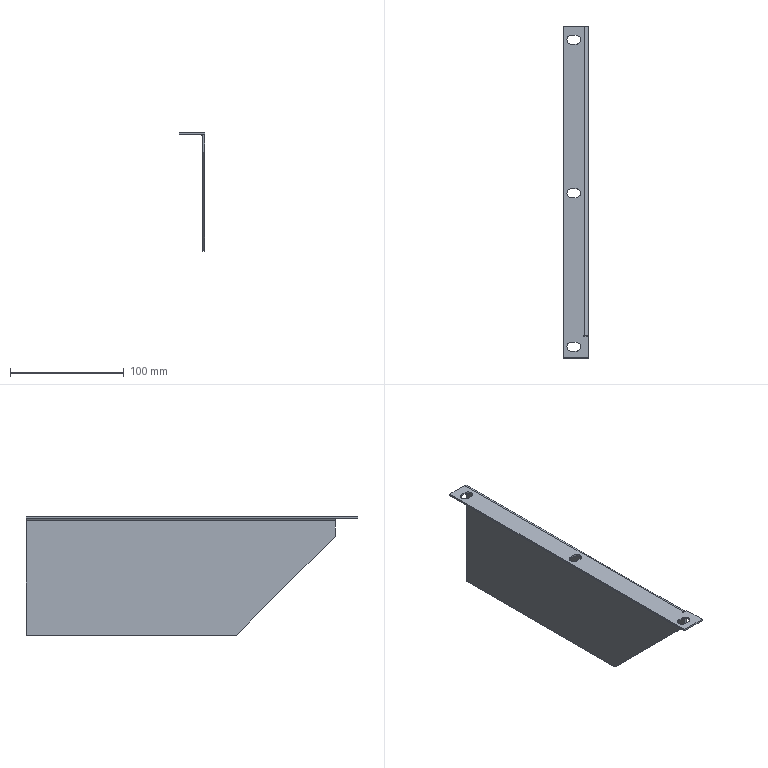Part | STEP file | SYL_0392D6J1SYL0380DJ100-657963 | 1 solid | 37 faces | box 22 x 292 x 104 mm | volume 44923 mm3 | plane 23 | cylinder 14 | commonest cylinder face diameters 8 x12 4 x1 7 x1
STEP:
#1=CARTESIAN_POINT('',(-13.5,120.,0.));
#2=VERTEX_POINT('',#1);
#3=CARTESIAN_POINT('',(-13.5,120.,-1.5));
#4=VERTEX_POINT('',#3);
#5=CARTESIAN_POINT('',(-13.5,120.,-1.5));
#6=DIRECTION('',(0.,0.,-1.));
#7=VECTOR('',#6,1000.);
#8=LINE('',#5,#7);
#9=EDGE_CURVE('',#2,#4,#8,.T.);
#10=ORIENTED_EDGE('',*,*,#9,.F.);
#11=CARTESIAN_POINT('',(-9.5,120.,0.));
#12=VERTEX_POINT('',#11);
#13=CARTESIAN_POINT('',(1.5,120.,0.));
#14=DIRECTION('',(1.,0.,0.));
#15=VECTOR('',#14,1000.);
#16=LINE('',#13,#15);
#17=EDGE_CURVE('',#2,#12,#16,.T.);
#18=ORIENTED_EDGE('',*,*,#17,.T.);
#19=CARTESIAN_POINT('',(-9.5,120.,-1.5));
#20=VERTEX_POINT('',#19);
#21=CARTESIAN_POINT('',(-9.5,120.,-1.5));
#22=DIRECTION('',(0.,0.,-1.));
#23=VECTOR('',#22,1000.);
#24=LINE('',#21,#23);
#25=EDGE_CURVE('',#12,#20,#24,.T.);
#26=ORIENTED_EDGE('',*,*,#25,.T.);
#27=CARTESIAN_POINT('',(-13.5,120.,-1.5));
#28=DIRECTION('',(1.,0.,0.));
#29=VECTOR('',#28,1000.);
#30=LINE('',#27,#29);
#31=EDGE_CURVE('',#4,#20,#30,.T.);
#32=ORIENTED_EDGE('',*,*,#31,.F.);
#33=EDGE_LOOP('',(#10,#18,#26,#32));
#34=FACE_OUTER_BOUND('',#33,.T.);
#35=CARTESIAN_POINT('',(-13.5,120.,-1.5));
#36=DIRECTION('',(0.,-1.,0.));
#37=DIRECTION('',(1.,0.,0.));
#38=AXIS2_PLACEMENT_3D('',#35,#36,#37);
#39=PLANE('',#38);
#40=ADVANCED_FACE('',(#34),#39,.F.);
#41=ORIENTED_EDGE('',*,*,#25,.F.);
#42=CARTESIAN_POINT('',(-5.5,124.,0.));
#43=VERTEX_POINT('',#42);
#44=CARTESIAN_POINT('',(-9.5,124.,0.));
#45=DIRECTION('',(0.,0.,1.));
#46=DIRECTION('',(1.,0.,0.));
#47=AXIS2_PLACEMENT_3D('',#44,#45,#46);
#48=CIRCLE('',#47,4.);
#49=EDGE_CURVE('',#12,#43,#48,.T.);
#50=ORIENTED_EDGE('',*,*,#49,.T.);
#51=CARTESIAN_POINT('',(-5.5,124.,-1.5));
#52=VERTEX_POINT('',#51);
#53=CARTESIAN_POINT('',(-5.5,124.,-1.5));
#54=DIRECTION('',(0.,0.,-1.));
#55=VECTOR('',#54,1000.);
#56=LINE('',#53,#55);
#57=EDGE_CURVE('',#43,#52,#56,.T.);
#58=ORIENTED_EDGE('',*,*,#57,.T.);
#59=CARTESIAN_POINT('',(-9.5,124.,-1.5));
#60=DIRECTION('',(0.,0.,1.));
#61=DIRECTION('',(0.,-1.,0.));
#62=AXIS2_PLACEMENT_3D('',#59,#60,#61);
#63=CIRCLE('',#62,4.);
#64=EDGE_CURVE('',#20,#52,#63,.T.);
#65=ORIENTED_EDGE('',*,*,#64,.F.);
#66=EDGE_LOOP('',(#41,#50,#58,#65));
#67=FACE_OUTER_BOUND('',#66,.T.);
#68=CARTESIAN_POINT('',(-9.5,124.,-1.5));
#69=DIRECTION('',(0.,0.,1.));
#70=DIRECTION('',(1.,0.,0.));
#71=AXIS2_PLACEMENT_3D('',#68,#69,#70);
#72=CYLINDRICAL_SURFACE('',#71,4.);
#73=ADVANCED_FACE('',(#67),#72,.F.);
#74=ORIENTED_EDGE('',*,*,#57,.F.);
#75=CARTESIAN_POINT('',(-9.5,128.,0.));
#76=VERTEX_POINT('',#75);
#77=CARTESIAN_POINT('',(-9.5,124.,0.));
#78=DIRECTION('',(0.,0.,1.));
#79=DIRECTION('',(1.,0.,0.));
#80=AXIS2_PLACEMENT_3D('',#77,#78,#79);
#81=CIRCLE('',#80,4.);
#82=EDGE_CURVE('',#43,#76,#81,.T.);
#83=ORIENTED_EDGE('',*,*,#82,.T.);
#84=CARTESIAN_POINT('',(-9.5,128.,-1.5));
#85=VERTEX_POINT('',#84);
#86=CARTESIAN_POINT('',(-9.5,128.,-1.5));
#87=DIRECTION('',(0.,0.,-1.));
#88=VECTOR('',#87,1000.);
#89=LINE('',#86,#88);
#90=EDGE_CURVE('',#76,#85,#89,.T.);
#91=ORIENTED_EDGE('',*,*,#90,.T.);
#92=CARTESIAN_POINT('',(-9.5,124.,-1.5));
#93=DIRECTION('',(0.,0.,1.));
#94=DIRECTION('',(1.,0.,0.));
#95=AXIS2_PLACEMENT_3D('',#92,#93,#94);
#96=CIRCLE('',#95,4.);
#97=EDGE_CURVE('',#52,#85,#96,.T.);
#98=ORIENTED_EDGE('',*,*,#97,.F.);
#99=EDGE_LOOP('',(#74,#83,#91,#98));
#100=FACE_OUTER_BOUND('',#99,.T.);
#101=CARTESIAN_POINT('',(-9.5,124.,-1.5));
#102=DIRECTION('',(0.,0.,1.));
#103=DIRECTION('',(1.,0.,0.));
#104=AXIS2_PLACEMENT_3D('',#101,#102,#103);
#105=CYLINDRICAL_SURFACE('',#104,4.);
#106=ADVANCED_FACE('',(#100),#105,.F.);
#107=ORIENTED_EDGE('',*,*,#90,.F.);
#108=CARTESIAN_POINT('',(-13.5,128.,0.));
#109=VERTEX_POINT('',#108);
#110=CARTESIAN_POINT('',(1.5,128.,0.));
#111=DIRECTION('',(-1.,0.,0.));
#112=VECTOR('',#111,1000.);
#113=LINE('',#110,#112);
#114=EDGE_CURVE('',#76,#109,#113,.T.);
#115=ORIENTED_EDGE('',*,*,#114,.T.);
#116=CARTESIAN_POINT('',(-13.5,128.,-1.5));
#117=VERTEX_POINT('',#116);
#118=CARTESIAN_POINT('',(-13.5,128.,-1.5));
#119=DIRECTION('',(0.,0.,-1.));
#120=VECTOR('',#119,1000.);
#121=LINE('',#118,#120);
#122=EDGE_CURVE('',#109,#117,#121,.T.);
#123=ORIENTED_EDGE('',*,*,#122,.T.);
#124=CARTESIAN_POINT('',(-9.5,128.,-1.5));
#125=DIRECTION('',(-1.,0.,0.));
#126=VECTOR('',#125,1000.);
#127=LINE('',#124,#126);
#128=EDGE_CURVE('',#85,#117,#127,.T.);
#129=ORIENTED_EDGE('',*,*,#128,.F.);
#130=EDGE_LOOP('',(#107,#115,#123,#129));
#131=FACE_OUTER_BOUND('',#130,.T.);
#132=CARTESIAN_POINT('',(-9.5,128.,-1.5));
#133=DIRECTION('',(0.,1.,0.));
#134=DIRECTION('',(-1.,0.,0.));
#135=AXIS2_PLACEMENT_3D('',#132,#133,#134);
#136=PLANE('',#135);
#137=ADVANCED_FACE('',(#131),#136,.F.);
#138=ORIENTED_EDGE('',*,*,#122,.F.);
#139=CARTESIAN_POINT('',(-17.5,124.,0.));
#140=VERTEX_POINT('',#139);
#141=CARTESIAN_POINT('',(-13.5,124.,0.));
#142=DIRECTION('',(0.,0.,1.));
#143=DIRECTION('',(1.,0.,0.));
#144=AXIS2_PLACEMENT_3D('',#141,#142,#143);
#145=CIRCLE('',#144,4.);
#146=EDGE_CURVE('',#109,#140,#145,.T.);
#147=ORIENTED_EDGE('',*,*,#146,.T.);
#148=CARTESIAN_POINT('',(-17.5,124.,-1.5));
#149=VERTEX_POINT('',#148);
#150=CARTESIAN_POINT('',(-17.5,124.,-1.5));
#151=DIRECTION('',(0.,0.,-1.));
#152=VECTOR('',#151,1000.);
#153=LINE('',#150,#152);
#154=EDGE_CURVE('',#140,#149,#153,.T.);
#155=ORIENTED_EDGE('',*,*,#154,.T.);
#156=CARTESIAN_POINT('',(-13.5,124.,-1.5));
#157=DIRECTION('',(0.,0.,1.));
#158=DIRECTION('',(0.,1.,0.));
#159=AXIS2_PLACEMENT_3D('',#156,#157,#158);
#160=CIRCLE('',#159,4.);
#161=EDGE_CURVE('',#117,#149,#160,.T.);
#162=ORIENTED_EDGE('',*,*,#161,.F.);
#163=EDGE_LOOP('',(#138,#147,#155,#162));
#164=FACE_OUTER_BOUND('',#163,.T.);
#165=CARTESIAN_POINT('',(-13.5,124.,-1.5));
#166=DIRECTION('',(0.,0.,1.));
#167=DIRECTION('',(1.,0.,0.));
#168=AXIS2_PLACEMENT_3D('',#165,#166,#167);
#169=CYLINDRICAL_SURFACE('',#168,4.);
#170=ADVANCED_FACE('',(#164),#169,.F.);
#171=CARTESIAN_POINT('',(-13.5,-15.,0.));
#172=VERTEX_POINT('',#171);
#173=CARTESIAN_POINT('',(-13.5,-15.,-1.5));
#174=VERTEX_POINT('',#173);
#175=CARTESIAN_POINT('',(-13.5,-15.,-1.5));
#176=DIRECTION('',(0.,0.,-1.));
#177=VECTOR('',#176,1000.);
#178=LINE('',#175,#177);
#179=EDGE_CURVE('',#172,#174,#178,.T.);
#180=ORIENTED_EDGE('',*,*,#179,.F.);
#181=CARTESIAN_POINT('',(-9.5,-15.,0.));
#182=VERTEX_POINT('',#181);
#183=CARTESIAN_POINT('',(1.5,-15.,0.));
#184=DIRECTION('',(1.,0.,0.));
#185=VECTOR('',#184,1000.);
#186=LINE('',#183,#185);
#187=EDGE_CURVE('',#172,#182,#186,.T.);
#188=ORIENTED_EDGE('',*,*,#187,.T.);
#189=CARTESIAN_POINT('',(-9.5,-15.,-1.5));
#190=VERTEX_POINT('',#189);
#191=CARTESIAN_POINT('',(-9.5,-15.,-1.5));
#192=DIRECTION('',(0.,0.,-1.));
#193=VECTOR('',#192,1000.);
#194=LINE('',#191,#193);
#195=EDGE_CURVE('',#182,#190,#194,.T.);
#196=ORIENTED_EDGE('',*,*,#195,.T.);
#197=CARTESIAN_POINT('',(-13.5,-15.,-1.5));
#198=DIRECTION('',(1.,0.,0.));
#199=VECTOR('',#198,1000.);
#200=LINE('',#197,#199);
#201=EDGE_CURVE('',#174,#190,#200,.T.);
#202=ORIENTED_EDGE('',*,*,#201,.F.);
#203=EDGE_LOOP('',(#180,#188,#196,#202));
#204=FACE_OUTER_BOUND('',#203,.T.);
#205=CARTESIAN_POINT('',(-13.5,-15.,-1.5));
#206=DIRECTION('',(0.,-1.,0.));
#207=DIRECTION('',(1.,0.,0.));
#208=AXIS2_PLACEMENT_3D('',#205,#206,#207);
#209=PLANE('',#208);
#210=ADVANCED_FACE('',(#204),#209,.F.);
#211=ORIENTED_EDGE('',*,*,#195,.F.);
#212=CARTESIAN_POINT('',(-5.5,-11.,0.));
#213=VERTEX_POINT('',#212);
#214=CARTESIAN_POINT('',(-9.5,-11.,0.));
#215=DIRECTION('',(0.,0.,1.));
#216=DIRECTION('',(1.,0.,0.));
#217=AXIS2_PLACEMENT_3D('',#214,#215,#216);
#218=CIRCLE('',#217,4.);
#219=EDGE_CURVE('',#182,#213,#218,.T.);
#220=ORIENTED_EDGE('',*,*,#219,.T.);
#221=CARTESIAN_POINT('',(-5.5,-11.,-1.5));
#222=VERTEX_POINT('',#221);
#223=CARTESIAN_POINT('',(-5.5,-11.,-1.5));
#224=DIRECTION('',(0.,0.,-1.));
#225=VECTOR('',#224,1000.);
#226=LINE('',#223,#225);
#227=EDGE_CURVE('',#213,#222,#226,.T.);
#228=ORIENTED_EDGE('',*,*,#227,.T.);
#229=CARTESIAN_POINT('',(-9.5,-11.,-1.5));
#230=DIRECTION('',(0.,0.,1.));
#231=DIRECTION('',(0.,-1.,0.));
#232=AXIS2_PLACEMENT_3D('',#229,#230,#231);
#233=CIRCLE('',#232,4.);
#234=EDGE_CURVE('',#190,#222,#233,.T.);
#235=ORIENTED_EDGE('',*,*,#234,.F.);
#236=EDGE_LOOP('',(#211,#220,#228,#235));
#237=FACE_OUTER_BOUND('',#236,.T.);
#238=CARTESIAN_POINT('',(-9.5,-11.,-1.5));
#239=DIRECTION('',(0.,0.,1.));
#240=DIRECTION('',(1.,0.,0.));
#241=AXIS2_PLACEMENT_3D('',#238,#239,#240);
#242=CYLINDRICAL_SURFACE('',#241,4.);
#243=ADVANCED_FACE('',(#237),#242,.F.);
#244=ORIENTED_EDGE('',*,*,#227,.F.);
#245=CARTESIAN_POINT('',(-9.5,-7.,0.));
#246=VERTEX_POINT('',#245);
#247=CARTESIAN_POINT('',(-9.5,-11.,0.));
#248=DIRECTION('',(0.,0.,1.));
#249=DIRECTION('',(1.,0.,0.));
#250=AXIS2_PLACEMENT_3D('',#247,#248,#249);
#251=CIRCLE('',#250,4.);
#252=EDGE_CURVE('',#213,#246,#251,.T.);
#253=ORIENTED_EDGE('',*,*,#252,.T.);
#254=CARTESIAN_POINT('',(-9.5,-7.,-1.5));
#255=VERTEX_POINT('',#254);
#256=CARTESIAN_POINT('',(-9.5,-7.,-1.5));
#257=DIRECTION('',(0.,0.,-1.));
#258=VECTOR('',#257,1000.);
#259=LINE('',#256,#258);
#260=EDGE_CURVE('',#246,#255,#259,.T.);
#261=ORIENTED_EDGE('',*,*,#260,.T.);
#262=CARTESIAN_POINT('',(-9.5,-11.,-1.5));
#263=DIRECTION('',(0.,0.,1.));
#264=DIRECTION('',(1.,0.,0.));
#265=AXIS2_PLACEMENT_3D('',#262,#263,#264);
#266=CIRCLE('',#265,4.);
#267=EDGE_CURVE('',#222,#255,#266,.T.);
#268=ORIENTED_EDGE('',*,*,#267,.F.);
#269=EDGE_LOOP('',(#244,#253,#261,#268));
#270=FACE_OUTER_BOUND('',#269,.T.);
#271=CARTESIAN_POINT('',(-9.5,-11.,-1.5));
#272=DIRECTION('',(0.,0.,1.));
#273=DIRECTION('',(1.,0.,0.));
#274=AXIS2_PLACEMENT_3D('',#271,#272,#273);
#275=CYLINDRICAL_SURFACE('',#274,4.);
#276=ADVANCED_FACE('',(#270),#275,.F.);
#277=ORIENTED_EDGE('',*,*,#260,.F.);
#278=CARTESIAN_POINT('',(-13.5,-7.,0.));
#279=VERTEX_POINT('',#278);
#280=CARTESIAN_POINT('',(1.5,-7.,0.));
#281=DIRECTION('',(-1.,0.,0.));
#282=VECTOR('',#281,1000.);
#283=LINE('',#280,#282);
#284=EDGE_CURVE('',#246,#279,#283,.T.);
#285=ORIENTED_EDGE('',*,*,#284,.T.);
#286=CARTESIAN_POINT('',(-13.5,-7.,-1.5));
#287=VERTEX_POINT('',#286);
#288=CARTESIAN_POINT('',(-13.5,-7.,-1.5));
#289=DIRECTION('',(0.,0.,-1.));
#290=VECTOR('',#289,1000.);
#291=LINE('',#288,#290);
#292=EDGE_CURVE('',#279,#287,#291,.T.);
#293=ORIENTED_EDGE('',*,*,#292,.T.);
#294=CARTESIAN_POINT('',(-9.5,-7.,-1.5));
#295=DIRECTION('',(-1.,0.,0.));
#296=VECTOR('',#295,1000.);
#297=LINE('',#294,#296);
#298=EDGE_CURVE('',#255,#287,#297,.T.);
#299=ORIENTED_EDGE('',*,*,#298,.F.);
#300=EDGE_LOOP('',(#277,#285,#293,#299));
#301=FACE_OUTER_BOUND('',#300,.T.);
#302=CARTESIAN_POINT('',(-9.5,-7.,-1.5));
#303=DIRECTION('',(0.,1.,0.));
#304=DIRECTION('',(-1.,0.,0.));
#305=AXIS2_PLACEMENT_3D('',#302,#303,#304);
#306=PLANE('',#305);
#307=ADVANCED_FACE('',(#301),#306,.F.);
#308=ORIENTED_EDGE('',*,*,#292,.F.);
#309=CARTESIAN_POINT('',(-17.5,-11.,0.));
#310=VERTEX_POINT('',#309);
#311=CARTESIAN_POINT('',(-13.5,-11.,0.));
#312=DIRECTION('',(0.,0.,1.));
#313=DIRECTION('',(1.,0.,0.));
#314=AXIS2_PLACEMENT_3D('',#311,#312,#313);
#315=CIRCLE('',#314,4.);
#316=EDGE_CURVE('',#279,#310,#315,.T.);
#317=ORIENTED_EDGE('',*,*,#316,.T.);
#318=CARTESIAN_POINT('',(-17.5,-11.,-1.5));
#319=VERTEX_POINT('',#318);
#320=CARTESIAN_POINT('',(-17.5,-11.,-1.5));
#321=DIRECTION('',(0.,0.,-1.));
#322=VECTOR('',#321,1000.);
#323=LINE('',#320,#322);
#324=EDGE_CURVE('',#310,#319,#323,.T.);
#325=ORIENTED_EDGE('',*,*,#324,.T.);
#326=CARTESIAN_POINT('',(-13.5,-11.,-1.5));
#327=DIRECTION('',(0.,0.,1.));
#328=DIRECTION('',(0.,1.,0.));
#329=AXIS2_PLACEMENT_3D('',#326,#327,#328);
#330=CIRCLE('',#329,4.);
#331=EDGE_CURVE('',#287,#319,#330,.T.);
#332=ORIENTED_EDGE('',*,*,#331,.F.);
#333=EDGE_LOOP('',(#308,#317,#325,#332));
#334=FACE_OUTER_BOUND('',#333,.T.);
#335=CARTESIAN_POINT('',(-13.5,-11.,-1.5));
#336=DIRECTION('',(0.,0.,1.));
#337=DIRECTION('',(1.,0.,0.));
#338=AXIS2_PLACEMENT_3D('',#335,#336,#337);
#339=CYLINDRICAL_SURFACE('',#338,4.);
#340=ADVANCED_FACE('',(#334),#339,.F.);
#341=CARTESIAN_POINT('',(-13.5,-150.,0.));
#342=VERTEX_POINT('',#341);
#343=CARTESIAN_POINT('',(-13.5,-150.,-1.5));
#344=VERTEX_POINT('',#343);
#345=CARTESIAN_POINT('',(-13.5,-150.,-1.5));
#346=DIRECTION('',(0.,0.,-1.));
#347=VECTOR('',#346,1000.);
#348=LINE('',#345,#347);
#349=EDGE_CURVE('',#342,#344,#348,.T.);
#350=ORIENTED_EDGE('',*,*,#349,.F.);
#351=CARTESIAN_POINT('',(-9.5,-150.,0.));
#352=VERTEX_POINT('',#351);
#353=CARTESIAN_POINT('',(1.5,-150.,0.));
#354=DIRECTION('',(1.,0.,0.));
#355=VECTOR('',#354,1000.);
#356=LINE('',#353,#355);
#357=EDGE_CURVE('',#342,#352,#356,.T.);
#358=ORIENTED_EDGE('',*,*,#357,.T.);
#359=CARTESIAN_POINT('',(-9.5,-150.,-1.5));
#360=VERTEX_POINT('',#359);
#361=CARTESIAN_POINT('',(-9.5,-150.,-1.5));
#362=DIRECTION('',(0.,0.,-1.));
#363=VECTOR('',#362,1000.);
#364=LINE('',#361,#363);
#365=EDGE_CURVE('',#352,#360,#364,.T.);
#366=ORIENTED_EDGE('',*,*,#365,.T.);
#367=CARTESIAN_POINT('',(-13.5,-150.,-1.5));
#368=DIRECTION('',(1.,0.,0.));
#369=VECTOR('',#368,1000.);
#370=LINE('',#367,#369);
#371=EDGE_CURVE('',#344,#360,#370,.T.);
#372=ORIENTED_EDGE('',*,*,#371,.F.);
#373=EDGE_LOOP('',(#350,#358,#366,#372));
#374=FACE_OUTER_BOUND('',#373,.T.);
#375=CARTESIAN_POINT('',(-13.5,-150.,-1.5));
#376=DIRECTION('',(0.,-1.,0.));
#377=DIRECTION('',(1.,0.,0.));
#378=AXIS2_PLACEMENT_3D('',#375,#376,#377);
#379=PLANE('',#378);
#380=ADVANCED_FACE('',(#374),#379,.F.);
#381=ORIENTED_EDGE('',*,*,#365,.F.);
#382=CARTESIAN_POINT('',(-5.5,-146.,0.));
#383=VERTEX_POINT('',#382);
#384=CARTESIAN_POINT('',(-9.5,-146.,0.));
#385=DIRECTION('',(0.,0.,1.));
#386=DIRECTION('',(1.,0.,0.));
#387=AXIS2_PLACEMENT_3D('',#384,#385,#386);
#388=CIRCLE('',#387,4.);
#389=EDGE_CURVE('',#352,#383,#388,.T.);
#390=ORIENTED_EDGE('',*,*,#389,.T.);
#391=CARTESIAN_POINT('',(-5.5,-146.,-1.5));
#392=VERTEX_POINT('',#391);
#393=CARTESIAN_POINT('',(-5.5,-146.,-1.5));
#394=DIRECTION('',(0.,0.,-1.));
#395=VECTOR('',#394,1000.);
#396=LINE('',#393,#395);
#397=EDGE_CURVE('',#383,#392,#396,.T.);
#398=ORIENTED_EDGE('',*,*,#397,.T.);
#399=CARTESIAN_POINT('',(-9.5,-146.,-1.5));
#400=DIRECTION('',(0.,0.,1.));
#401=DIRECTION('',(0.,-1.,0.));
#402=AXIS2_PLACEMENT_3D('',#399,#400,#401);
#403=CIRCLE('',#402,4.);
#404=EDGE_CURVE('',#360,#392,#403,.T.);
#405=ORIENTED_EDGE('',*,*,#404,.F.);
#406=EDGE_LOOP('',(#381,#390,#398,#405));
#407=FACE_OUTER_BOUND('',#406,.T.);
#408=CARTESIAN_POINT('',(-9.5,-146.,-1.5));
#409=DIRECTION('',(0.,0.,1.));
#410=DIRECTION('',(1.,0.,0.));
#411=AXIS2_PLACEMENT_3D('',#408,#409,#410);
#412=CYLINDRICAL_SURFACE('',#411,4.);
#413=ADVANCED_FACE('',(#407),#412,.F.);
#414=ORIENTED_EDGE('',*,*,#397,.F.);
#415=CARTESIAN_POINT('',(-9.5,-142.,0.));
#416=VERTEX_POINT('',#415);
#417=CARTESIAN_POINT('',(-9.5,-146.,0.));
#418=DIRECTION('',(0.,0.,1.));
#419=DIRECTION('',(1.,0.,0.));
#420=AXIS2_PLACEMENT_3D('',#417,#418,#419);
#421=CIRCLE('',#420,4.);
#422=EDGE_CURVE('',#383,#416,#421,.T.);
#423=ORIENTED_EDGE('',*,*,#422,.T.);
#424=CARTESIAN_POINT('',(-9.5,-142.,-1.5));
#425=VERTEX_POINT('',#424);
#426=CARTESIAN_POINT('',(-9.5,-142.,-1.5));
#427=DIRECTION('',(0.,0.,-1.));
#428=VECTOR('',#427,1000.);
#429=LINE('',#426,#428);
#430=EDGE_CURVE('',#416,#425,#429,.T.);
#431=ORIENTED_EDGE('',*,*,#430,.T.);
#432=CARTESIAN_POINT('',(-9.5,-146.,-1.5));
#433=DIRECTION('',(0.,0.,1.));
#434=DIRECTION('',(1.,0.,0.));
#435=AXIS2_PLACEMENT_3D('',#432,#433,#434);
#436=CIRCLE('',#435,4.);
#437=EDGE_CURVE('',#392,#425,#436,.T.);
#438=ORIENTED_EDGE('',*,*,#437,.F.);
#439=EDGE_LOOP('',(#414,#423,#431,#438));
#440=FACE_OUTER_BOUND('',#439,.T.);
#441=CARTESIAN_POINT('',(-9.5,-146.,-1.5));
#442=DIRECTION('',(0.,0.,1.));
#443=DIRECTION('',(1.,0.,0.));
#444=AXIS2_PLACEMENT_3D('',#441,#442,#443);
#445=CYLINDRICAL_SURFACE('',#444,4.);
#446=ADVANCED_FACE('',(#440),#445,.F.);
#447=ORIENTED_EDGE('',*,*,#430,.F.);
#448=CARTESIAN_POINT('',(-13.5,-142.,0.));
#449=VERTEX_POINT('',#448);
#450=CARTESIAN_POINT('',(1.5,-142.,0.));
#451=DIRECTION('',(-1.,0.,0.));
#452=VECTOR('',#451,1000.);
#453=LINE('',#450,#452);
#454=EDGE_CURVE('',#416,#449,#453,.T.);
#455=ORIENTED_EDGE('',*,*,#454,.T.);
#456=CARTESIAN_POINT('',(-13.5,-142.,-1.5));
#457=VERTEX_POINT('',#456);
#458=CARTESIAN_POINT('',(-13.5,-142.,-1.5));
#459=DIRECTION('',(0.,0.,-1.));
#460=VECTOR('',#459,1000.);
#461=LINE('',#458,#460);
#462=EDGE_CURVE('',#449,#457,#461,.T.);
#463=ORIENTED_EDGE('',*,*,#462,.T.);
#464=CARTESIAN_POINT('',(-9.5,-142.,-1.5));
#465=DIRECTION('',(-1.,0.,0.));
#466=VECTOR('',#465,1000.);
#467=LINE('',#464,#466);
#468=EDGE_CURVE('',#425,#457,#467,.T.);
#469=ORIENTED_EDGE('',*,*,#468,.F.);
#470=EDGE_LOOP('',(#447,#455,#463,#469));
#471=FACE_OUTER_BOUND('',#470,.T.);
#472=CARTESIAN_POINT('',(-9.5,-142.,-1.5));
#473=DIRECTION('',(0.,1.,0.));
#474=DIRECTION('',(-1.,0.,0.));
#475=AXIS2_PLACEMENT_3D('',#472,#473,#474);
#476=PLANE('',#475);
#477=ADVANCED_FACE('',(#471),#476,.F.);
#478=ORIENTED_EDGE('',*,*,#462,.F.);
#479=CARTESIAN_POINT('',(-17.5,-146.,0.));
#480=VERTEX_POINT('',#479);
#481=CARTESIAN_POINT('',(-13.5,-146.,0.));
#482=DIRECTION('',(0.,0.,1.));
#483=DIRECTION('',(1.,0.,0.));
#484=AXIS2_PLACEMENT_3D('',#481,#482,#483);
#485=CIRCLE('',#484,4.);
#486=EDGE_CURVE('',#449,#480,#485,.T.);
#487=ORIENTED_EDGE('',*,*,#486,.T.);
#488=CARTESIAN_POINT('',(-17.5,-146.,-1.5));
#489=VERTEX_POINT('',#488);
#490=CARTESIAN_POINT('',(-17.5,-146.,-1.5));
#491=DIRECTION('',(0.,0.,-1.));
#492=VECTOR('',#491,1000.);
#493=LINE('',#490,#492);
#494=EDGE_CURVE('',#480,#489,#493,.T.);
#495=ORIENTED_EDGE('',*,*,#494,.T.);
#496=CARTESIAN_POINT('',(-13.5,-146.,-1.5));
#497=DIRECTION('',(0.,0.,1.));
#498=DIRECTION('',(0.,1.,0.));
#499=AXIS2_PLACEMENT_3D('',#496,#497,#498);
#500=CIRCLE('',#499,4.);
#501=EDGE_CURVE('',#457,#489,#500,.T.);
#502=ORIENTED_EDGE('',*,*,#501,.F.);
#503=EDGE_LOOP('',(#478,#487,#495,#502));
#504=FACE_OUTER_BOUND('',#503,.T.);
#505=CARTESIAN_POINT('',(-13.5,-146.,-1.5));
#506=DIRECTION('',(0.,0.,1.));
#507=DIRECTION('',(1.,0.,0.));
#508=AXIS2_PLACEMENT_3D('',#505,#506,#507);
#509=CYLINDRICAL_SURFACE('',#508,4.);
#510=ADVANCED_FACE('',(#504),#509,.F.);
#511=CARTESIAN_POINT('',(-2.75,-136.,0.));
#512=VERTEX_POINT('',#511);
#513=CARTESIAN_POINT('',(-2.75,-136.,-1.5));
#514=VERTEX_POINT('',#513);
#515=CARTESIAN_POINT('',(-2.75,-136.,-1.5));
#516=DIRECTION('',(0.,0.,-1.));
#517=VECTOR('',#516,1000.);
#518=LINE('',#515,#517);
#519=EDGE_CURVE('',#512,#514,#518,.T.);
#520=ORIENTED_EDGE('',*,*,#519,.F.);
#521=CARTESIAN_POINT('',(-2.75,-136.75,0.));
#522=VERTEX_POINT('',#521);
#523=CARTESIAN_POINT('',(-2.75,71.373,0.));
#524=DIRECTION('',(0.,-1.,0.));
#525=VECTOR('',#524,1000.);
#526=LINE('',#523,#525);
#527=EDGE_CURVE('',#512,#522,#526,.T.);
#528=ORIENTED_EDGE('',*,*,#527,.T.);
#529=CARTESIAN_POINT('',(-2.75,-136.75,-1.5));
#530=VERTEX_POINT('',#529);
#531=CARTESIAN_POINT('',(-2.75,-136.75,-1.5));
#532=DIRECTION('',(0.,0.,-1.));
#533=VECTOR('',#532,1000.);
#534=LINE('',#531,#533);
#535=EDGE_CURVE('',#522,#530,#534,.T.);
#536=ORIENTED_EDGE('',*,*,#535,.T.);
#537=CARTESIAN_POINT('',(-2.75,71.373,-1.5));
#538=DIRECTION('',(0.,-1.,0.));
#539=VECTOR('',#538,1000.);
#540=LINE('',#537,#539);
#541=EDGE_CURVE('',#514,#530,#540,.T.);
#542=ORIENTED_EDGE('',*,*,#541,.F.);
#543=EDGE_LOOP('',(#520,#528,#536,#542));
#544=FACE_OUTER_BOUND('',#543,.T.);
#545=CARTESIAN_POINT('',(-2.75,71.373,-1.5));
#546=DIRECTION('',(-1.,0.,0.));
#547=DIRECTION('',(0.,-1.,0.));
#548=AXIS2_PLACEMENT_3D('',#545,#546,#547);
#549=PLANE('',#548);
#550=ADVANCED_FACE('',(#544),#549,.F.);
#551=ORIENTED_EDGE('',*,*,#535,.F.);
#552=CARTESIAN_POINT('',(1.5,-136.75,0.));
#553=VERTEX_POINT('',#552);
#554=CARTESIAN_POINT('',(1.5,-136.75,0.));
#555=DIRECTION('',(1.,0.,0.));
#556=VECTOR('',#555,1000.);
#557=LINE('',#554,#556);
#558=EDGE_CURVE('',#522,#553,#557,.T.);
#559=ORIENTED_EDGE('',*,*,#558,.T.);
#560=CARTESIAN_POINT('',(1.5,-136.75,-1.5));
#561=VERTEX_POINT('',#560);
#562=CARTESIAN_POINT('',(1.5,-136.75,-1.5));
#563=DIRECTION('',(0.,0.,-1.));
#564=VECTOR('',#563,1000.);
#565=LINE('',#562,#564);
#566=EDGE_CURVE('',#553,#561,#565,.T.);
#567=ORIENTED_EDGE('',*,*,#566,.T.);
#568=CARTESIAN_POINT('',(1.5,-136.75,-1.5));
#569=DIRECTION('',(1.,0.,0.));
#570=VECTOR('',#569,1000.);
#571=LINE('',#568,#570);
#572=EDGE_CURVE('',#530,#561,#571,.T.);
#573=ORIENTED_EDGE('',*,*,#572,.F.);
#574=EDGE_LOOP('',(#551,#559,#567,#573));
#575=FACE_OUTER_BOUND('',#574,.T.);
#576=CARTESIAN_POINT('',(1.5,-136.75,-1.5));
#577=DIRECTION('',(0.,-1.,0.));
#578=DIRECTION('',(1.,0.,0.));
#579=AXIS2_PLACEMENT_3D('',#576,#577,#578);
#580=PLANE('',#579);
#581=ADVANCED_FACE('',(#575),#580,.F.);
#582=ORIENTED_EDGE('',*,*,#566,.F.);
#583=CARTESIAN_POINT('',(1.5,-156.,0.));
#584=VERTEX_POINT('',#583);
#585=CARTESIAN_POINT('',(1.5,71.373,0.));
#586=DIRECTION('',(0.,-1.,0.));
#587=VECTOR('',#586,1000.);
#588=LINE('',#585,#587);
#589=EDGE_CURVE('',#553,#584,#588,.T.);
#590=ORIENTED_EDGE('',*,*,#589,.T.);
#591=CARTESIAN_POINT('',(1.5,-156.,-1.5));
#592=VERTEX_POINT('',#591);
#593=CARTESIAN_POINT('',(1.5,-156.,-1.5));
#594=DIRECTION('',(0.,0.,-1.));
#595=VECTOR('',#594,1000.);
#596=LINE('',#593,#595);
#597=EDGE_CURVE('',#584,#592,#596,.T.);
#598=ORIENTED_EDGE('',*,*,#597,.T.);
#599=CARTESIAN_POINT('',(1.5,-136.,-1.5));
#600=DIRECTION('',(0.,-1.,0.));
#601=VECTOR('',#600,1000.);
#602=LINE('',#599,#601);
#603=EDGE_CURVE('',#561,#592,#602,.T.);
#604=ORIENTED_EDGE('',*,*,#603,.F.);
#605=EDGE_LOOP('',(#582,#590,#598,#604));
#606=FACE_OUTER_BOUND('',#605,.T.);
#607=CARTESIAN_POINT('',(1.5,-136.,-1.5));
#608=DIRECTION('',(-1.,0.,0.));
#609=DIRECTION('',(0.,-1.,0.));
#610=AXIS2_PLACEMENT_3D('',#607,#608,#609);
#611=PLANE('',#610);
#612=ADVANCED_FACE('',(#606),#611,.F.);
#613=ORIENTED_EDGE('',*,*,#597,.F.);
#614=CARTESIAN_POINT('',(-20.5,-156.,0.));
#615=VERTEX_POINT('',#614);
#616=CARTESIAN_POINT('',(1.5,-156.,0.));
#617=DIRECTION('',(-1.,0.,0.));
#618=VECTOR('',#617,1000.);
#619=LINE('',#616,#618);
#620=EDGE_CURVE('',#584,#615,#619,.T.);
#621=ORIENTED_EDGE('',*,*,#620,.T.);
#622=CARTESIAN_POINT('',(-20.5,-156.,-1.5));
#623=VERTEX_POINT('',#622);
#624=CARTESIAN_POINT('',(-20.5,-156.,-1.5));
#625=DIRECTION('',(0.,0.,-1.));
#626=VECTOR('',#625,1000.);
#627=LINE('',#624,#626);
#628=EDGE_CURVE('',#615,#623,#627,.T.);
#629=ORIENTED_EDGE('',*,*,#628,.T.);
#630=CARTESIAN_POINT('',(1.5,-156.,-1.5));
#631=DIRECTION('',(-1.,0.,0.));
#632=VECTOR('',#631,1000.);
#633=LINE('',#630,#632);
#634=EDGE_CURVE('',#592,#623,#633,.T.);
#635=ORIENTED_EDGE('',*,*,#634,.F.);
#636=EDGE_LOOP('',(#613,#621,#629,#635));
#637=FACE_OUTER_BOUND('',#636,.T.);
#638=CARTESIAN_POINT('',(1.5,-156.,-1.5));
#639=DIRECTION('',(0.,1.,0.));
#640=DIRECTION('',(-1.,0.,0.));
#641=AXIS2_PLACEMENT_3D('',#638,#639,#640);
#642=PLANE('',#641);
#643=ADVANCED_FACE('',(#637),#642,.F.);
#644=ORIENTED_EDGE('',*,*,#628,.F.);
#645=CARTESIAN_POINT('',(-20.5,136.,0.));
#646=VERTEX_POINT('',#645);
#647=CARTESIAN_POINT('',(-20.5,71.373,0.));
#648=DIRECTION('',(0.,1.,0.));
#649=VECTOR('',#648,1000.);
#650=LINE('',#647,#649);
#651=EDGE_CURVE('',#615,#646,#650,.T.);
#652=ORIENTED_EDGE('',*,*,#651,.T.);
#653=CARTESIAN_POINT('',(-20.5,136.,-1.5));
#654=VERTEX_POINT('',#653);
#655=CARTESIAN_POINT('',(-20.5,136.,-1.5));
#656=DIRECTION('',(0.,0.,-1.));
#657=VECTOR('',#656,1000.);
#658=LINE('',#655,#657);
#659=EDGE_CURVE('',#646,#654,#658,.T.);
#660=ORIENTED_EDGE('',*,*,#659,.T.);
#661=CARTESIAN_POINT('',(-20.5,-156.,-1.5));
#662=DIRECTION('',(0.,1.,0.));
#663=VECTOR('',#662,1000.);
#664=LINE('',#661,#663);
#665=EDGE_CURVE('',#623,#654,#664,.T.);
#666=ORIENTED_EDGE('',*,*,#665,.F.);
#667=EDGE_LOOP('',(#644,#652,#660,#666));
#668=FACE_OUTER_BOUND('',#667,.T.);
#669=CARTESIAN_POINT('',(-20.5,-156.,-1.5));
#670=DIRECTION('',(1.,0.,0.));
#671=DIRECTION('',(0.,1.,0.));
#672=AXIS2_PLACEMENT_3D('',#669,#670,#671);
#673=PLANE('',#672);
#674=ADVANCED_FACE('',(#668),#673,.F.);
#675=ORIENTED_EDGE('',*,*,#659,.F.);
#676=CARTESIAN_POINT('',(-2.,136.,0.));
#677=VERTEX_POINT('',#676);
#678=CARTESIAN_POINT('',(1.5,136.,0.));
#679=DIRECTION('',(1.,0.,0.));
#680=VECTOR('',#679,1000.);
#681=LINE('',#678,#680);
#682=EDGE_CURVE('',#646,#677,#681,.T.);
#683=ORIENTED_EDGE('',*,*,#682,.T.);
#684=CARTESIAN_POINT('',(-2.,136.,-1.5));
#685=VERTEX_POINT('',#684);
#686=CARTESIAN_POINT('',(-2.,136.,-1.5));
#687=DIRECTION('',(0.,0.,-1.));
#688=VECTOR('',#687,1000.);
#689=LINE('',#686,#688);
#690=EDGE_CURVE('',#677,#685,#689,.T.);
#691=ORIENTED_EDGE('',*,*,#690,.T.);
#692=CARTESIAN_POINT('',(-20.5,136.,-1.5));
#693=DIRECTION('',(1.,0.,0.));
#694=VECTOR('',#693,1000.);
#695=LINE('',#692,#694);
#696=EDGE_CURVE('',#654,#685,#695,.T.);
#697=ORIENTED_EDGE('',*,*,#696,.F.);
#698=EDGE_LOOP('',(#675,#683,#691,#697));
#699=FACE_OUTER_BOUND('',#698,.T.);
#700=CARTESIAN_POINT('',(-20.5,136.,-1.5));
#701=DIRECTION('',(0.,-1.,0.));
#702=DIRECTION('',(1.,0.,0.));
#703=AXIS2_PLACEMENT_3D('',#700,#701,#702);
#704=PLANE('',#703);
#705=ADVANCED_FACE('',(#699),#704,.F.);
#706=ORIENTED_EDGE('',*,*,#690,.F.);
#707=CARTESIAN_POINT('',(1.5,136.,-3.5));
#708=VERTEX_POINT('',#707);
#709=CARTESIAN_POINT('',(-2.,136.,-3.5));
#710=DIRECTION('',(0.,-1.,0.));
#711=DIRECTION('',(0.,0.,1.));
#712=AXIS2_PLACEMENT_3D('',#709,#710,#711);
#713=CIRCLE('',#712,3.5);
#714=EDGE_CURVE('',#708,#677,#713,.T.);
#715=ORIENTED_EDGE('',*,*,#714,.F.);
#716=CARTESIAN_POINT('',(0.,136.,-3.5));
#717=VERTEX_POINT('',#716);
#718=CARTESIAN_POINT('',(0.,136.,-3.5));
#719=DIRECTION('',(-1.,0.,0.));
#720=VECTOR('',#719,1000.);
#721=LINE('',#718,#720);
#722=EDGE_CURVE('',#708,#717,#721,.T.);
#723=ORIENTED_EDGE('',*,*,#722,.T.);
#724=CARTESIAN_POINT('',(-2.,136.,-3.5));
#725=DIRECTION('',(0.,-1.,0.));
#726=DIRECTION('',(1.,0.,0.));
#727=AXIS2_PLACEMENT_3D('',#724,#725,#726);
#728=CIRCLE('',#727,2.);
#729=EDGE_CURVE('',#717,#685,#728,.T.);
#730=ORIENTED_EDGE('',*,*,#729,.T.);
#731=EDGE_LOOP('',(#706,#715,#723,#730));
#732=FACE_OUTER_BOUND('',#731,.T.);
#733=CARTESIAN_POINT('',(-2.,136.,-3.5));
#734=DIRECTION('',(0.,1.,0.));
#735=DIRECTION('',(0.,0.,1.));
#736=AXIS2_PLACEMENT_3D('',#733,#734,#735);
#737=PLANE('',#736);
#738=ADVANCED_FACE('',(#732),#737,.T.);
#739=ORIENTED_EDGE('',*,*,#722,.F.);
#740=CARTESIAN_POINT('',(1.5,136.,-104.));
#741=VERTEX_POINT('',#740);
#742=CARTESIAN_POINT('',(1.5,136.,0.));
#743=DIRECTION('',(0.,0.,-1.));
#744=VECTOR('',#743,1000.);
#745=LINE('',#742,#744);
#746=EDGE_CURVE('',#708,#741,#745,.T.);
#747=ORIENTED_EDGE('',*,*,#746,.T.);
#748=CARTESIAN_POINT('',(0.,136.,-104.));
#749=VERTEX_POINT('',#748);
#750=CARTESIAN_POINT('',(0.,136.,-104.));
#751=DIRECTION('',(-1.,0.,0.));
#752=VECTOR('',#751,1000.);
#753=LINE('',#750,#752);
#754=EDGE_CURVE('',#741,#749,#753,.T.);
#755=ORIENTED_EDGE('',*,*,#754,.T.);
#756=CARTESIAN_POINT('',(0.,136.,-3.5));
#757=DIRECTION('',(0.,0.,-1.));
#758=VECTOR('',#757,1000.);
#759=LINE('',#756,#758);
#760=EDGE_CURVE('',#717,#749,#759,.T.);
#761=ORIENTED_EDGE('',*,*,#760,.F.);
#762=EDGE_LOOP('',(#739,#747,#755,#761));
#763=FACE_OUTER_BOUND('',#762,.T.);
#764=CARTESIAN_POINT('',(0.,136.,-3.5));
#765=DIRECTION('',(0.,-1.,0.));
#766=DIRECTION('',(0.,0.,-1.));
#767=AXIS2_PLACEMENT_3D('',#764,#765,#766);
#768=PLANE('',#767);
#769=ADVANCED_FACE('',(#763),#768,.F.);
#770=ORIENTED_EDGE('',*,*,#754,.F.);
#771=CARTESIAN_POINT('',(1.5,-49.,-104.));
#772=VERTEX_POINT('',#771);
#773=CARTESIAN_POINT('',(1.5,0.,-104.));
#774=DIRECTION('',(0.,-1.,0.));
#775=VECTOR('',#774,1000.);
#776=LINE('',#773,#775);
#777=EDGE_CURVE('',#741,#772,#776,.T.);
#778=ORIENTED_EDGE('',*,*,#777,.T.);
#779=CARTESIAN_POINT('',(0.,-49.,-104.));
#780=VERTEX_POINT('',#779);
#781=CARTESIAN_POINT('',(0.,-49.,-104.));
#782=DIRECTION('',(-1.,0.,0.));
#783=VECTOR('',#782,1000.);
#784=LINE('',#781,#783);
#785=EDGE_CURVE('',#772,#780,#784,.T.);
#786=ORIENTED_EDGE('',*,*,#785,.T.);
#787=CARTESIAN_POINT('',(0.,136.,-104.));
#788=DIRECTION('',(0.,-1.,0.));
#789=VECTOR('',#788,1000.);
#790=LINE('',#787,#789);
#791=EDGE_CURVE('',#749,#780,#790,.T.);
#792=ORIENTED_EDGE('',*,*,#791,.F.);
#793=EDGE_LOOP('',(#770,#778,#786,#792));
#794=FACE_OUTER_BOUND('',#793,.T.);
#795=CARTESIAN_POINT('',(0.,136.,-104.));
#796=DIRECTION('',(0.,0.,1.));
#797=DIRECTION('',(0.,-1.,0.));
#798=AXIS2_PLACEMENT_3D('',#795,#796,#797);
#799=PLANE('',#798);
#800=ADVANCED_FACE('',(#794),#799,.F.);
#801=ORIENTED_EDGE('',*,*,#785,.F.);
#802=CARTESIAN_POINT('',(1.5,-136.,-17.));
#803=VERTEX_POINT('',#802);
#804=CARTESIAN_POINT('',(1.5,-49.,-104.));
#805=DIRECTION('',(0.,-0.7071,0.7071));
#806=VECTOR('',#805,1000.);
#807=LINE('',#804,#806);
#808=EDGE_CURVE('',#772,#803,#807,.T.);
#809=ORIENTED_EDGE('',*,*,#808,.T.);
#810=CARTESIAN_POINT('',(0.,-136.,-17.));
#811=VERTEX_POINT('',#810);
#812=CARTESIAN_POINT('',(0.,-136.,-17.));
#813=DIRECTION('',(-1.,0.,0.));
#814=VECTOR('',#813,1000.);
#815=LINE('',#812,#814);
#816=EDGE_CURVE('',#803,#811,#815,.T.);
#817=ORIENTED_EDGE('',*,*,#816,.T.);
#818=CARTESIAN_POINT('',(0.,-49.,-104.));
#819=DIRECTION('',(0.,-0.7071,0.7071));
#820=VECTOR('',#819,1000.);
#821=LINE('',#818,#820);
#822=EDGE_CURVE('',#780,#811,#821,.T.);
#823=ORIENTED_EDGE('',*,*,#822,.F.);
#824=EDGE_LOOP('',(#801,#809,#817,#823));
#825=FACE_OUTER_BOUND('',#824,.T.);
#826=CARTESIAN_POINT('',(0.,-49.,-104.));
#827=DIRECTION('',(0.,0.7071,0.7071));
#828=DIRECTION('',(0.,-0.7071,0.7071));
#829=AXIS2_PLACEMENT_3D('',#826,#827,#828);
#830=PLANE('',#829);
#831=ADVANCED_FACE('',(#825),#830,.F.);
#832=ORIENTED_EDGE('',*,*,#816,.F.);
#833=CARTESIAN_POINT('',(1.5,-136.,-3.5));
#834=VERTEX_POINT('',#833);
#835=CARTESIAN_POINT('',(1.5,-136.,0.));
#836=DIRECTION('',(0.,0.,1.));
#837=VECTOR('',#836,1000.);
#838=LINE('',#835,#837);
#839=EDGE_CURVE('',#803,#834,#838,.T.);
#840=ORIENTED_EDGE('',*,*,#839,.T.);
#841=CARTESIAN_POINT('',(0.,-136.,-3.5));
#842=VERTEX_POINT('',#841);
#843=CARTESIAN_POINT('',(0.,-136.,-3.5));
#844=DIRECTION('',(-1.,0.,0.));
#845=VECTOR('',#844,1000.);
#846=LINE('',#843,#845);
#847=EDGE_CURVE('',#834,#842,#846,.T.);
#848=ORIENTED_EDGE('',*,*,#847,.T.);
#849=CARTESIAN_POINT('',(0.,-136.,-17.));
#850=DIRECTION('',(0.,0.,1.));
#851=VECTOR('',#850,1000.);
#852=LINE('',#849,#851);
#853=EDGE_CURVE('',#811,#842,#852,.T.);
#854=ORIENTED_EDGE('',*,*,#853,.F.);
#855=EDGE_LOOP('',(#832,#840,#848,#854));
#856=FACE_OUTER_BOUND('',#855,.T.);
#857=CARTESIAN_POINT('',(0.,-136.,-17.));
#858=DIRECTION('',(0.,1.,0.));
#859=DIRECTION('',(0.,0.,1.));
#860=AXIS2_PLACEMENT_3D('',#857,#858,#859);
#861=PLANE('',#860);
#862=ADVANCED_FACE('',(#856),#861,.F.);
#863=ORIENTED_EDGE('',*,*,#847,.F.);
#864=CARTESIAN_POINT('',(-2.,-136.,0.));
#865=VERTEX_POINT('',#864);
#866=CARTESIAN_POINT('',(-2.,-136.,-3.5));
#867=DIRECTION('',(0.,1.,0.));
#868=DIRECTION('',(0.,0.,1.));
#869=AXIS2_PLACEMENT_3D('',#866,#867,#868);
#870=CIRCLE('',#869,3.5);
#871=EDGE_CURVE('',#865,#834,#870,.T.);
#872=ORIENTED_EDGE('',*,*,#871,.F.);
#873=CARTESIAN_POINT('',(-2.,-136.,-1.5));
#874=VERTEX_POINT('',#873);
#875=CARTESIAN_POINT('',(-2.,-136.,-1.5));
#876=DIRECTION('',(0.,0.,-1.));
#877=VECTOR('',#876,1000.);
#878=LINE('',#875,#877);
#879=EDGE_CURVE('',#865,#874,#878,.T.);
#880=ORIENTED_EDGE('',*,*,#879,.T.);
#881=CARTESIAN_POINT('',(-2.,-136.,-3.5));
#882=DIRECTION('',(0.,1.,0.));
#883=DIRECTION('',(0.,0.,1.));
#884=AXIS2_PLACEMENT_3D('',#881,#882,#883);
#885=CIRCLE('',#884,2.);
#886=EDGE_CURVE('',#874,#842,#885,.T.);
#887=ORIENTED_EDGE('',*,*,#886,.T.);
#888=EDGE_LOOP('',(#863,#872,#880,#887));
#889=FACE_OUTER_BOUND('',#888,.T.);
#890=CARTESIAN_POINT('',(-2.,-136.,-3.5));
#891=DIRECTION('',(0.,-1.,0.));
#892=DIRECTION('',(0.,0.,-1.));
#893=AXIS2_PLACEMENT_3D('',#890,#891,#892);
#894=PLANE('',#893);
#895=ADVANCED_FACE('',(#889),#894,.T.);
#896=CARTESIAN_POINT('',(-13.5,-146.,0.));
#897=DIRECTION('',(0.,0.,1.));
#898=DIRECTION('',(1.,0.,0.));
#899=AXIS2_PLACEMENT_3D('',#896,#897,#898);
#900=CIRCLE('',#899,4.);
#901=EDGE_CURVE('',#480,#342,#900,.T.);
#902=ORIENTED_EDGE('',*,*,#901,.T.);
#903=ORIENTED_EDGE('',*,*,#349,.T.);
#904=CARTESIAN_POINT('',(-13.5,-146.,-1.5));
#905=DIRECTION('',(0.,0.,1.));
#906=DIRECTION('',(-1.,0.,0.));
#907=AXIS2_PLACEMENT_3D('',#904,#905,#906);
#908=CIRCLE('',#907,4.);
#909=EDGE_CURVE('',#489,#344,#908,.T.);
#910=ORIENTED_EDGE('',*,*,#909,.F.);
#911=ORIENTED_EDGE('',*,*,#494,.F.);
#912=EDGE_LOOP('',(#902,#903,#910,#911));
#913=FACE_OUTER_BOUND('',#912,.T.);
#914=CARTESIAN_POINT('',(-13.5,-146.,-1.5));
#915=DIRECTION('',(0.,0.,1.));
#916=DIRECTION('',(1.,0.,0.));
#917=AXIS2_PLACEMENT_3D('',#914,#915,#916);
#918=CYLINDRICAL_SURFACE('',#917,4.);
#919=ADVANCED_FACE('',(#913),#918,.F.);
#920=CARTESIAN_POINT('',(-13.5,-11.,0.));
#921=DIRECTION('',(0.,0.,1.));
#922=DIRECTION('',(1.,0.,0.));
#923=AXIS2_PLACEMENT_3D('',#920,#921,#922);
#924=CIRCLE('',#923,4.);
#925=EDGE_CURVE('',#310,#172,#924,.T.);
#926=ORIENTED_EDGE('',*,*,#925,.T.);
#927=ORIENTED_EDGE('',*,*,#179,.T.);
#928=CARTESIAN_POINT('',(-13.5,-11.,-1.5));
#929=DIRECTION('',(0.,0.,1.));
#930=DIRECTION('',(-1.,0.,0.));
#931=AXIS2_PLACEMENT_3D('',#928,#929,#930);
#932=CIRCLE('',#931,4.);
#933=EDGE_CURVE('',#319,#174,#932,.T.);
#934=ORIENTED_EDGE('',*,*,#933,.F.);
#935=ORIENTED_EDGE('',*,*,#324,.F.);
#936=EDGE_LOOP('',(#926,#927,#934,#935));
#937=FACE_OUTER_BOUND('',#936,.T.);
#938=CARTESIAN_POINT('',(-13.5,-11.,-1.5));
#939=DIRECTION('',(0.,0.,1.));
#940=DIRECTION('',(1.,0.,0.));
#941=AXIS2_PLACEMENT_3D('',#938,#939,#940);
#942=CYLINDRICAL_SURFACE('',#941,4.);
#943=ADVANCED_FACE('',(#937),#942,.F.);
#944=CARTESIAN_POINT('',(-13.5,124.,0.));
#945=DIRECTION('',(0.,0.,1.));
#946=DIRECTION('',(1.,0.,0.));
#947=AXIS2_PLACEMENT_3D('',#944,#945,#946);
#948=CIRCLE('',#947,4.);
#949=EDGE_CURVE('',#140,#2,#948,.T.);
#950=ORIENTED_EDGE('',*,*,#949,.T.);
#951=ORIENTED_EDGE('',*,*,#9,.T.);
#952=CARTESIAN_POINT('',(-13.5,124.,-1.5));
#953=DIRECTION('',(0.,0.,1.));
#954=DIRECTION('',(-1.,0.,0.));
#955=AXIS2_PLACEMENT_3D('',#952,#953,#954);
#956=CIRCLE('',#955,4.);
#957=EDGE_CURVE('',#149,#4,#956,.T.);
#958=ORIENTED_EDGE('',*,*,#957,.F.);
#959=ORIENTED_EDGE('',*,*,#154,.F.);
#960=EDGE_LOOP('',(#950,#951,#958,#959));
#961=FACE_OUTER_BOUND('',#960,.T.);
#962=CARTESIAN_POINT('',(-13.5,124.,-1.5));
#963=DIRECTION('',(0.,0.,1.));
#964=DIRECTION('',(1.,0.,0.));
#965=AXIS2_PLACEMENT_3D('',#962,#963,#964);
#966=CYLINDRICAL_SURFACE('',#965,4.);
#967=ADVANCED_FACE('',(#961),#966,.F.);
#968=CARTESIAN_POINT('',(1.5,-136.,0.));
#969=DIRECTION('',(-1.,0.,0.));
#970=VECTOR('',#969,1000.);
#971=LINE('',#968,#970);
#972=EDGE_CURVE('',#865,#512,#971,.T.);
#973=ORIENTED_EDGE('',*,*,#972,.T.);
#974=ORIENTED_EDGE('',*,*,#519,.T.);
#975=CARTESIAN_POINT('',(1.5,-136.,-1.5));
#976=DIRECTION('',(-1.,0.,0.));
#977=VECTOR('',#976,1000.);
#978=LINE('',#975,#977);
#979=EDGE_CURVE('',#874,#514,#978,.T.);
#980=ORIENTED_EDGE('',*,*,#979,.F.);
#981=ORIENTED_EDGE('',*,*,#879,.F.);
#982=EDGE_LOOP('',(#973,#974,#980,#981));
#983=FACE_OUTER_BOUND('',#982,.T.);
#984=CARTESIAN_POINT('',(1.5,-136.,-1.5));
#985=DIRECTION('',(0.,1.,0.));
#986=DIRECTION('',(-1.,0.,0.));
#987=AXIS2_PLACEMENT_3D('',#984,#985,#986);
#988=PLANE('',#987);
#989=ADVANCED_FACE('',(#983),#988,.F.);
#990=ORIENTED_EDGE('',*,*,#886,.F.);
#991=CARTESIAN_POINT('',(-2.,-136.,-1.5));
#992=DIRECTION('',(0.,1.,0.));
#993=VECTOR('',#992,1000.);
#994=LINE('',#991,#993);
#995=EDGE_CURVE('',#874,#685,#994,.T.);
#996=ORIENTED_EDGE('',*,*,#995,.T.);
#997=ORIENTED_EDGE('',*,*,#729,.F.);
#998=CARTESIAN_POINT('',(0.,136.,-3.5));
#999=DIRECTION('',(0.,-1.,0.));
#1000=VECTOR('',#999,1000.);
#1001=LINE('',#998,#1000);
#1002=EDGE_CURVE('',#717,#842,#1001,.T.);
#1003=ORIENTED_EDGE('',*,*,#1002,.T.);
#1004=EDGE_LOOP('',(#990,#996,#997,#1003));
#1005=FACE_OUTER_BOUND('',#1004,.T.);
#1006=CARTESIAN_POINT('',(-2.,-136.,-3.5));
#1007=DIRECTION('',(0.,1.,0.));
#1008=DIRECTION('',(0.,0.,1.));
#1009=AXIS2_PLACEMENT_3D('',#1006,#1007,#1008);
#1010=CYLINDRICAL_SURFACE('',#1009,2.);
#1011=ADVANCED_FACE('',(#1005),#1010,.F.);
#1012=ORIENTED_EDGE('',*,*,#822,.T.);
#1013=ORIENTED_EDGE('',*,*,#853,.T.);
#1014=ORIENTED_EDGE('',*,*,#1002,.F.);
#1015=ORIENTED_EDGE('',*,*,#760,.T.);
#1016=ORIENTED_EDGE('',*,*,#791,.T.);
#1017=EDGE_LOOP('',(#1012,#1013,#1014,#1015,#1016));
#1018=FACE_OUTER_BOUND('',#1017,.T.);
#1019=CARTESIAN_POINT('',(0.,0.,0.));
#1020=DIRECTION('',(1.,0.,0.));
#1021=DIRECTION('',(0.,1.,0.));
#1022=AXIS2_PLACEMENT_3D('',#1019,#1020,#1021);
#1023=PLANE('',#1022);
#1024=ADVANCED_FACE('',(#1018),#1023,.F.);
#1025=ORIENTED_EDGE('',*,*,#995,.F.);
#1026=ORIENTED_EDGE('',*,*,#979,.T.);
#1027=ORIENTED_EDGE('',*,*,#541,.T.);
#1028=ORIENTED_EDGE('',*,*,#572,.T.);
#1029=ORIENTED_EDGE('',*,*,#603,.T.);
#1030=ORIENTED_EDGE('',*,*,#634,.T.);
#1031=ORIENTED_EDGE('',*,*,#665,.T.);
#1032=ORIENTED_EDGE('',*,*,#696,.T.);
#1033=EDGE_LOOP('',(#1025,#1026,#1027,#1028,#1029,#1030,#1031,#1032));
#1034=FACE_OUTER_BOUND('',#1033,.T.);
#1035=ORIENTED_EDGE('',*,*,#501,.T.);
#1036=ORIENTED_EDGE('',*,*,#909,.T.);
#1037=ORIENTED_EDGE('',*,*,#371,.T.);
#1038=ORIENTED_EDGE('',*,*,#404,.T.);
#1039=ORIENTED_EDGE('',*,*,#437,.T.);
#1040=ORIENTED_EDGE('',*,*,#468,.T.);
#1041=EDGE_LOOP('',(#1035,#1036,#1037,#1038,#1039,#1040));
#1042=FACE_BOUND('',#1041,.T.);
#1043=ORIENTED_EDGE('',*,*,#331,.T.);
#1044=ORIENTED_EDGE('',*,*,#933,.T.);
#1045=ORIENTED_EDGE('',*,*,#201,.T.);
#1046=ORIENTED_EDGE('',*,*,#234,.T.);
#1047=ORIENTED_EDGE('',*,*,#267,.T.);
#1048=ORIENTED_EDGE('',*,*,#298,.T.);
#1049=EDGE_LOOP('',(#1043,#1044,#1045,#1046,#1047,#1048));
#1050=FACE_BOUND('',#1049,.T.);
#1051=ORIENTED_EDGE('',*,*,#161,.T.);
#1052=ORIENTED_EDGE('',*,*,#957,.T.);
#1053=ORIENTED_EDGE('',*,*,#31,.T.);
#1054=ORIENTED_EDGE('',*,*,#64,.T.);
#1055=ORIENTED_EDGE('',*,*,#97,.T.);
#1056=ORIENTED_EDGE('',*,*,#128,.T.);
#1057=EDGE_LOOP('',(#1051,#1052,#1053,#1054,#1055,#1056));
#1058=FACE_BOUND('',#1057,.T.);
#1059=CARTESIAN_POINT('',(1.5,71.373,-1.5));
#1060=DIRECTION('',(0.,0.,1.));
#1061=DIRECTION('',(1.,0.,0.));
#1062=AXIS2_PLACEMENT_3D('',#1059,#1060,#1061);
#1063=PLANE('',#1062);
#1064=ADVANCED_FACE('',(#1034,#1042,#1050,#1058),#1063,.F.);
#1065=ORIENTED_EDGE('',*,*,#871,.T.);
#1066=CARTESIAN_POINT('',(1.5,-136.,-3.5));
#1067=DIRECTION('',(0.,-1.,0.));
#1068=VECTOR('',#1067,1000.);
#1069=LINE('',#1066,#1068);
#1070=EDGE_CURVE('',#708,#834,#1069,.T.);
#1071=ORIENTED_EDGE('',*,*,#1070,.F.);
#1072=ORIENTED_EDGE('',*,*,#714,.T.);
#1073=CARTESIAN_POINT('',(-2.,-136.,0.));
#1074=DIRECTION('',(0.,1.,0.));
#1075=VECTOR('',#1074,1000.);
#1076=LINE('',#1073,#1075);
#1077=EDGE_CURVE('',#865,#677,#1076,.T.);
#1078=ORIENTED_EDGE('',*,*,#1077,.F.);
#1079=EDGE_LOOP('',(#1065,#1071,#1072,#1078));
#1080=FACE_OUTER_BOUND('',#1079,.T.);
#1081=CARTESIAN_POINT('',(-2.,-136.,-3.5));
#1082=DIRECTION('',(0.,1.,0.));
#1083=DIRECTION('',(0.,0.,1.));
#1084=AXIS2_PLACEMENT_3D('',#1081,#1082,#1083);
#1085=CYLINDRICAL_SURFACE('',#1084,3.5);
#1086=ADVANCED_FACE('',(#1080),#1085,.T.);
#1087=ORIENTED_EDGE('',*,*,#808,.F.);
#1088=ORIENTED_EDGE('',*,*,#777,.F.);
#1089=ORIENTED_EDGE('',*,*,#746,.F.);
#1090=ORIENTED_EDGE('',*,*,#1070,.T.);
#1091=ORIENTED_EDGE('',*,*,#839,.F.);
#1092=EDGE_LOOP('',(#1087,#1088,#1089,#1090,#1091));
#1093=FACE_OUTER_BOUND('',#1092,.T.);
#1094=CARTESIAN_POINT('',(1.5,0.,0.));
#1095=DIRECTION('',(1.,0.,0.));
#1096=DIRECTION('',(0.,1.,0.));
#1097=AXIS2_PLACEMENT_3D('',#1094,#1095,#1096);
#1098=PLANE('',#1097);
#1099=ADVANCED_FACE('',(#1093),#1098,.T.);
#1100=ORIENTED_EDGE('',*,*,#1077,.T.);
#1101=ORIENTED_EDGE('',*,*,#682,.F.);
#1102=ORIENTED_EDGE('',*,*,#651,.F.);
#1103=ORIENTED_EDGE('',*,*,#620,.F.);
#1104=ORIENTED_EDGE('',*,*,#589,.F.);
#1105=ORIENTED_EDGE('',*,*,#558,.F.);
#1106=ORIENTED_EDGE('',*,*,#527,.F.);
#1107=ORIENTED_EDGE('',*,*,#972,.F.);
#1108=EDGE_LOOP('',(#1100,#1101,#1102,#1103,#1104,#1105,#1106,#1107));
#1109=FACE_OUTER_BOUND('',#1108,.T.);
#1110=ORIENTED_EDGE('',*,*,#486,.F.);
#1111=ORIENTED_EDGE('',*,*,#454,.F.);
#1112=ORIENTED_EDGE('',*,*,#422,.F.);
#1113=ORIENTED_EDGE('',*,*,#389,.F.);
#1114=ORIENTED_EDGE('',*,*,#357,.F.);
#1115=ORIENTED_EDGE('',*,*,#901,.F.);
#1116=EDGE_LOOP('',(#1110,#1111,#1112,#1113,#1114,#1115));
#1117=FACE_BOUND('',#1116,.T.);
#1118=ORIENTED_EDGE('',*,*,#316,.F.);
#1119=ORIENTED_EDGE('',*,*,#284,.F.);
#1120=ORIENTED_EDGE('',*,*,#252,.F.);
#1121=ORIENTED_EDGE('',*,*,#219,.F.);
#1122=ORIENTED_EDGE('',*,*,#187,.F.);
#1123=ORIENTED_EDGE('',*,*,#925,.F.);
#1124=EDGE_LOOP('',(#1118,#1119,#1120,#1121,#1122,#1123));
#1125=FACE_BOUND('',#1124,.T.);
#1126=ORIENTED_EDGE('',*,*,#146,.F.);
#1127=ORIENTED_EDGE('',*,*,#114,.F.);
#1128=ORIENTED_EDGE('',*,*,#82,.F.);
#1129=ORIENTED_EDGE('',*,*,#49,.F.);
#1130=ORIENTED_EDGE('',*,*,#17,.F.);
#1131=ORIENTED_EDGE('',*,*,#949,.F.);
#1132=EDGE_LOOP('',(#1126,#1127,#1128,#1129,#1130,#1131));
#1133=FACE_BOUND('',#1132,.T.);
#1134=CARTESIAN_POINT('',(1.5,71.373,0.));
#1135=DIRECTION('',(0.,0.,1.));
#1136=DIRECTION('',(1.,0.,0.));
#1137=AXIS2_PLACEMENT_3D('',#1134,#1135,#1136);
#1138=PLANE('',#1137);
#1139=ADVANCED_FACE('',(#1109,#1117,#1125,#1133),#1138,.T.);
#1140=CLOSED_SHELL('',(#40,#73,#106,#137,#170,#210,#243,#276,#307,#340,#380,#413,#446,#477,#510,#550,#581,#612,#643,#674,#705,#738,#769,#800,#831,#862,#895,#919,#943,#967,#989,#1011,#1024,#1064,#1086,#1099,#1139));
#1141=MANIFOLD_SOLID_BREP('',#1140);
#1142=CARTESIAN_POINT('',(0.,0.,0.));
#1143=DIRECTION('',(0.,0.,1.));
#1144=DIRECTION('',(1.,0.,0.));
#1145=AXIS2_PLACEMENT_3D('',#1142,#1143,#1144);
#1146=(LENGTH_UNIT()NAMED_UNIT(*)SI_UNIT(.MILLI.,.METRE.));
#1147=UNCERTAINTY_MEASURE_WITH_UNIT(LENGTH_MEASURE(0.00001),#1146,'','');
#1148=(NAMED_UNIT(*)PLANE_ANGLE_UNIT()SI_UNIT($,.RADIAN.));
#1149=(NAMED_UNIT(*)SI_UNIT($,.STERADIAN.)SOLID_ANGLE_UNIT());
#1150=(GEOMETRIC_REPRESENTATION_CONTEXT(3)GLOBAL_UNCERTAINTY_ASSIGNED_CONTEXT((#1147))GLOBAL_UNIT_ASSIGNED_CONTEXT((#1146,#1148,#1149))REPRESENTATION_CONTEXT('',''));
#1151=ADVANCED_BREP_SHAPE_REPRESENTATION('',(#1141,#1145),#1150);